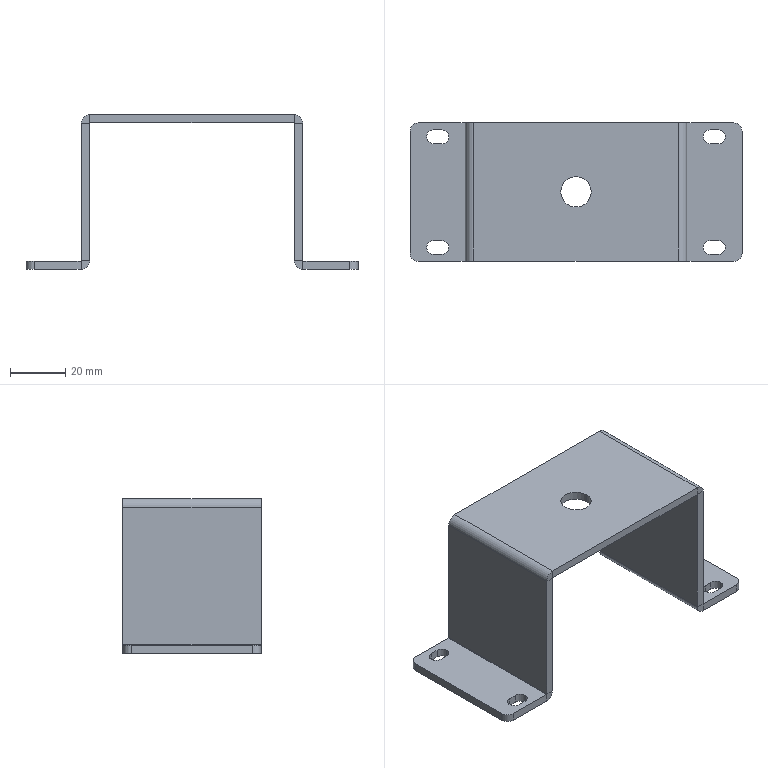Part | SolidWorks | features EdgeFlange 3, ICE 2, Fillet 1, FlatPattern 1, SMBaseFlange 1, SheetMetal 1 | 1 solid | 64 faces | box 120 x 50 x 56 mm | volume 32764 mm3 | plane 38 | cylinder 26 | commonest cylinder face diameters 5 x12 0.2 x4 6 x4 6.2 x4 11 x2